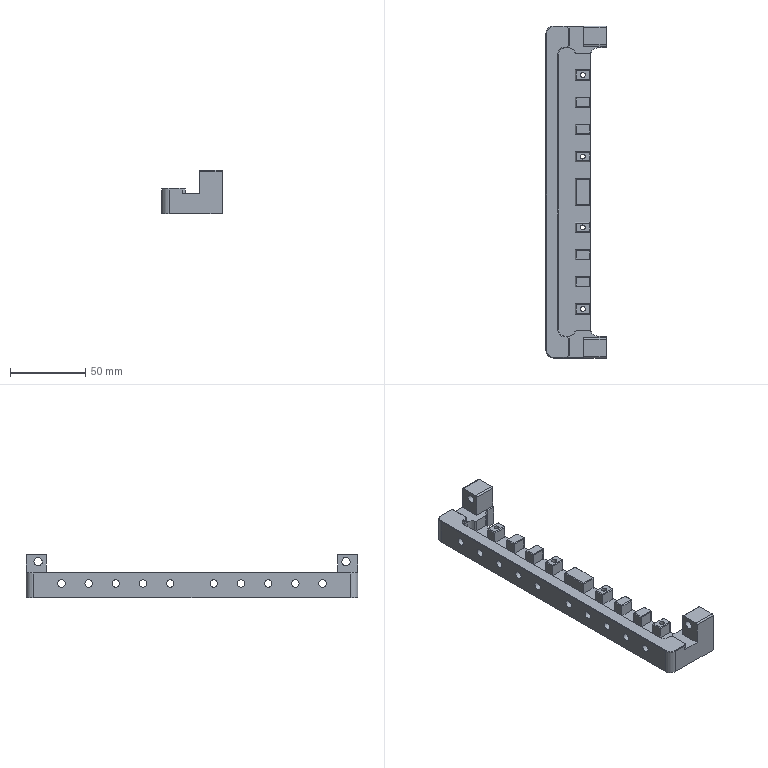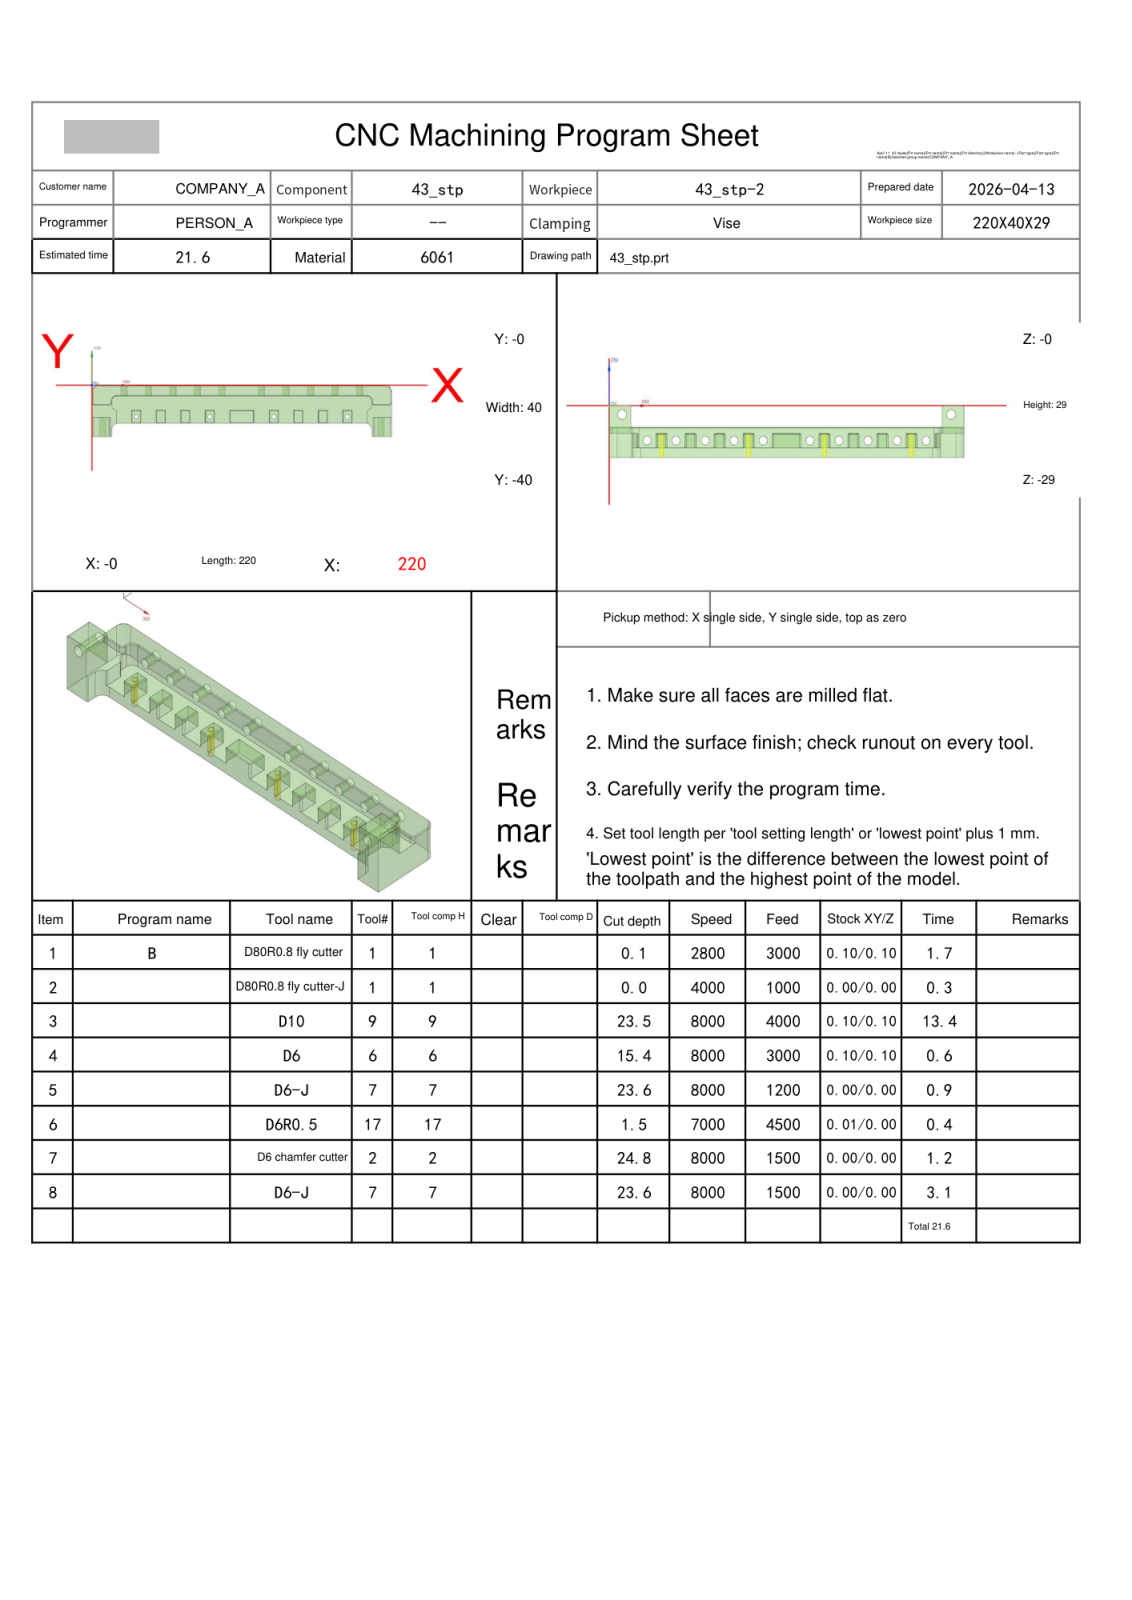NC program | NX | posted by the shop | part box 40 x 220 x 29 mm
Lines 8431 to 9376 of 14837:
N5 T07 M06
(D6-J  D=6. R=0. H=07 ce=0.00 di=0.00)
G00 G90 G54 X201.901 Y-14.131 M03 S8000
G43 H07 Z20.
M08
Z-12.147
G01 X201.908 Y-14.129 Z-12.238 F1200.
X201.93 Y-14.122 Z-12.32
X201.963 Y-14.111 Z-12.393
X202.006 Y-14.095 Z-12.458
X202.056 Y-14.074 Z-12.516
X202.112 Y-14.047 Z-12.565
X202.17 Y-14.014 Z-12.608
X202.23 Y-13.975 Z-12.644
X202.289 Y-13.929 Z-12.674
X202.345 Y-13.877 Z-12.698
X202.395 Y-13.817 Z-12.717
X202.438 Y-13.75 Z-12.73
X202.471 Y-13.675 Z-12.74
X202.492 Y-13.592 Z-12.745
X202.5 Y-13.5 Z-12.747
Y-12.5
G03 X201.5 Y-11.5 I-1. J0.0
G01 X200.434
X200.355 Y-11.516 Z-12.748
X200.299 Y-11.561 Z-12.75
X200.263 Y-11.632 Z-12.754
X200.246 Y-11.723 Z-12.76
X200.247 Y-11.833 Z-12.767
X200.263 Y-11.955 Z-12.774
X200.293 Y-12.087 Z-12.783
X200.336 Y-12.224 Z-12.793
X200.39 Y-12.363 Z-12.803
X200.453 Y-12.5 Z-12.813
X200.602 Y-12.754 Z-12.836
X200.78 Y-12.982 Z-12.858
X200.987 Y-13.183 Z-12.882
X201.221 Y-13.355 Z-12.904
X201.482 Y-13.498 Z-12.927
X201.621 Y-13.558 Z-12.937
X201.763 Y-13.609 Z-12.947
X201.903 Y-13.649 Z-12.957
X202.037 Y-13.677 Z-12.966
X202.162 Y-13.691 Z-12.973
X202.273 Y-13.69 Z-12.98
X202.366 Y-13.672 Z-12.986
X202.438 Y-13.635 Z-12.99
X202.484 Y-13.579 Z-12.992
X202.5 Y-13.5 Z-12.993
Y-12.5
G03 X201.5 Y-11.5 I-1. J0.0
G01 X200.434
X200.355 Y-11.516 Z-12.994
X200.299 Y-11.561 Z-12.997
X200.263 Y-11.632 Z-13.001
X200.246 Y-11.723 Z-13.006
X200.247 Y-11.833 Z-13.013
X200.263 Y-11.955 Z-13.021
X200.293 Y-12.087 Z-13.03
X200.336 Y-12.224 Z-13.039
X200.39 Y-12.363 Z-13.05
X200.453 Y-12.5 Z-13.06
X200.602 Y-12.754 Z-13.082
X200.78 Y-12.982 Z-13.105
X200.987 Y-13.183 Z-13.128
X201.221 Y-13.355 Z-13.151
X201.482 Y-13.498 Z-13.173
X201.621 Y-13.558 Z-13.184
X201.763 Y-13.609 Z-13.194
X201.903 Y-13.649 Z-13.203
X202.037 Y-13.677 Z-13.212
X202.162 Y-13.691 Z-13.22
X202.273 Y-13.69 Z-13.227
X202.366 Y-13.672 Z-13.232
X202.438 Y-13.635 Z-13.237
X202.484 Y-13.579 Z-13.239
X202.5 Y-13.5 Z-13.24
Y-12.5
G03 X201.5 Y-11.5 I-1. J0.0
G01 X200.434
X200.355 Y-11.516 Z-13.241
X200.299 Y-11.561 Z-13.243
X200.263 Y-11.632 Z-13.248
X200.246 Y-11.723 Z-13.253
X200.247 Y-11.833 Z-13.26
X200.263 Y-11.955 Z-13.268
X200.293 Y-12.087 Z-13.277
X200.336 Y-12.224 Z-13.286
X200.39 Y-12.363 Z-13.296
X200.453 Y-12.5 Z-13.307
X200.602 Y-12.754 Z-13.329
X200.78 Y-12.982 Z-13.352
X200.987 Y-13.183 Z-13.375
X201.221 Y-13.355 Z-13.398
X201.482 Y-13.498 Z-13.42
X201.621 Y-13.558 Z-13.43
X201.763 Y-13.609 Z-13.441
X201.903 Y-13.649 Z-13.45
X202.037 Y-13.677 Z-13.459
X202.162 Y-13.692 Z-13.467
X202.273 Y-13.69 Z-13.474
X202.366 Y-13.672 Z-13.479
X202.438 Y-13.635 Z-13.483
X202.484 Y-13.579 Z-13.486
X202.5 Y-13.5 Z-13.487
Y-12.5
G03 X201.5 Y-11.5 I-1. J0.0
G01 X200.434
X200.355 Y-11.516 Z-13.488
X200.299 Y-11.561 Z-13.49
X200.263 Y-11.632 Z-13.494
X200.246 Y-11.723 Z-13.5
X200.247 Y-11.833 Z-13.507
X200.263 Y-11.955 Z-13.514
X200.293 Y-12.087 Z-13.523
X200.336 Y-12.224 Z-13.533
X200.39 Y-12.363 Z-13.543
X200.453 Y-12.5 Z-13.553
X200.602 Y-12.754 Z-13.576
X200.78 Y-12.982 Z-13.598
X200.987 Y-13.183 Z-13.622
X201.221 Y-13.355 Z-13.644
X201.482 Y-13.498 Z-13.667
X201.621 Y-13.558 Z-13.677
X201.763 Y-13.609 Z-13.687
X201.903 Y-13.649 Z-13.697
X202.037 Y-13.677 Z-13.706
X202.162 Y-13.692 Z-13.713
X202.273 Y-13.69 Z-13.72
X202.366 Y-13.672 Z-13.726
X202.438 Y-13.635 Z-13.73
X202.484 Y-13.579 Z-13.732
X202.5 Y-13.5 Z-13.733
Y-12.5
G03 X201.5 Y-11.5 I-1. J0.0
G01 X200.434
X200.355 Y-11.516 Z-13.734
X200.299 Y-11.561 Z-13.737
X200.263 Y-11.632 Z-13.741
X200.246 Y-11.723 Z-13.746
X200.247 Y-11.833 Z-13.753
X200.263 Y-11.955 Z-13.761
X200.293 Y-12.087 Z-13.77
X200.336 Y-12.224 Z-13.779
X200.39 Y-12.363 Z-13.79
X200.453 Y-12.5 Z-13.8
X200.602 Y-12.754 Z-13.822
X200.78 Y-12.982 Z-13.845
X200.987 Y-13.183 Z-13.868
X201.221 Y-13.355 Z-13.891
X201.482 Y-13.498 Z-13.913
X201.621 Y-13.558 Z-13.924
X201.763 Y-13.609 Z-13.934
X201.903 Y-13.649 Z-13.943
X202.037 Y-13.677 Z-13.952
X202.162 Y-13.692 Z-13.96
X202.273 Y-13.69 Z-13.967
X202.366 Y-13.672 Z-13.972
X202.438 Y-13.635 Z-13.977
X202.484 Y-13.579 Z-13.979
X202.5 Y-13.5 Z-13.98
Y-12.5
G03 X201.5 Y-11.5 I-1. J0.0
G01 X200.434
X200.355 Y-11.516 Z-13.981
X200.299 Y-11.561 Z-13.983
X200.263 Y-11.632 Z-13.988
X200.246 Y-11.723 Z-13.993
X200.247 Y-11.833 Z-14.
X200.263 Y-11.955 Z-14.008
X200.293 Y-12.087 Z-14.017
X200.336 Y-12.224 Z-14.026
X200.39 Y-12.363 Z-14.036
X200.453 Y-12.5 Z-14.047
X200.602 Y-12.754 Z-14.069
X200.78 Y-12.982 Z-14.092
X200.987 Y-13.183 Z-14.115
X201.221 Y-13.355 Z-14.138
X201.482 Y-13.498 Z-14.16
X201.621 Y-13.558 Z-14.17
X201.763 Y-13.609 Z-14.181
X201.903 Y-13.649 Z-14.19
X202.037 Y-13.677 Z-14.199
X202.162 Y-13.692 Z-14.207
X202.273 Y-13.69 Z-14.214
X202.366 Y-13.672 Z-14.219
X202.438 Y-13.635 Z-14.223
X202.484 Y-13.579 Z-14.226
X202.5 Y-13.5 Z-14.227
Y-12.5
G03 X201.5 Y-11.5 I-1. J0.0
G01 X200.434
X200.355 Y-11.516 Z-14.228
X200.299 Y-11.561 Z-14.23
X200.263 Y-11.632 Z-14.234
X200.246 Y-11.723 Z-14.24
X200.247 Y-11.833 Z-14.247
X200.263 Y-11.955 Z-14.254
X200.293 Y-12.087 Z-14.263
X200.336 Y-12.224 Z-14.273
X200.39 Y-12.363 Z-14.283
X200.453 Y-12.5 Z-14.293
X200.602 Y-12.754 Z-14.316
X200.78 Y-12.982 Z-14.338
X200.987 Y-13.183 Z-14.362
X201.221 Y-13.355 Z-14.384
X201.482 Y-13.498 Z-14.407
X201.621 Y-13.558 Z-14.417
X201.763 Y-13.609 Z-14.427
X201.903 Y-13.649 Z-14.437
X202.037 Y-13.677 Z-14.446
X202.162 Y-13.692 Z-14.453
X202.273 Y-13.69 Z-14.46
X202.366 Y-13.672 Z-14.466
X202.438 Y-13.635 Z-14.47
X202.484 Y-13.579 Z-14.472
X202.5 Y-13.5 Z-14.473
Y-12.5
G03 X201.5 Y-11.5 I-1. J0.0
G01 X200.434
X200.355 Y-11.516 Z-14.474
X200.299 Y-11.561 Z-14.477
X200.263 Y-11.632 Z-14.481
X200.246 Y-11.723 Z-14.486
X200.247 Y-11.833 Z-14.493
X200.263 Y-11.955 Z-14.501
X200.293 Y-12.087 Z-14.51
X200.336 Y-12.224 Z-14.519
X200.39 Y-12.363 Z-14.53
X200.453 Y-12.5 Z-14.54
X200.602 Y-12.754 Z-14.562
X200.78 Y-12.982 Z-14.585
X200.987 Y-13.183 Z-14.608
X201.221 Y-13.355 Z-14.631
X201.482 Y-13.498 Z-14.653
X201.621 Y-13.558 Z-14.664
X201.763 Y-13.609 Z-14.674
X201.903 Y-13.649 Z-14.683
X202.037 Y-13.677 Z-14.692
X202.162 Y-13.692 Z-14.7
X202.273 Y-13.69 Z-14.707
X202.366 Y-13.672 Z-14.712
X202.438 Y-13.635 Z-14.717
X202.484 Y-13.579 Z-14.719
X202.5 Y-13.5 Z-14.72
Y-12.5
G03 X201.5 Y-11.5 I-1. J0.0
G01 X200.434
X200.355 Y-11.516 Z-14.721
X200.299 Y-11.561 Z-14.723
X200.263 Y-11.632 Z-14.728
X200.246 Y-11.723 Z-14.733
X200.247 Y-11.833 Z-14.74
X200.263 Y-11.955 Z-14.748
X200.293 Y-12.087 Z-14.757
X200.336 Y-12.224 Z-14.766
X200.39 Y-12.363 Z-14.776
X200.453 Y-12.5 Z-14.787
X200.602 Y-12.754 Z-14.809
X200.78 Y-12.982 Z-14.832
X200.987 Y-13.183 Z-14.855
X201.221 Y-13.355 Z-14.878
X201.482 Y-13.498 Z-14.9
X201.621 Y-13.558 Z-14.91
X201.763 Y-13.609 Z-14.921
X201.903 Y-13.649 Z-14.93
X202.037 Y-13.677 Z-14.939
X202.162 Y-13.692 Z-14.947
X202.273 Y-13.69 Z-14.954
X202.366 Y-13.672 Z-14.959
X202.438 Y-13.635 Z-14.963
X202.484 Y-13.579 Z-14.966
X202.5 Y-13.5 Z-14.967
Y-12.5
G03 X201.5 Y-11.5 I-1. J0.0
G01 X200.434
X200.355 Y-11.516 Z-14.968
X200.299 Y-11.561 Z-14.97
X200.263 Y-11.632 Z-14.974
X200.246 Y-11.723 Z-14.98
X200.247 Y-11.833 Z-14.987
X200.263 Y-11.955 Z-14.994
X200.293 Y-12.087 Z-15.003
X200.336 Y-12.224 Z-15.013
X200.39 Y-12.363 Z-15.023
X200.453 Y-12.5 Z-15.033
X200.602 Y-12.754 Z-15.056
X200.78 Y-12.982 Z-15.078
X200.987 Y-13.183 Z-15.102
X201.221 Y-13.355 Z-15.124
X201.482 Y-13.498 Z-15.147
X201.621 Y-13.558 Z-15.157
X201.763 Y-13.609 Z-15.167
X201.903 Y-13.649 Z-15.177
X202.037 Y-13.677 Z-15.186
X202.162 Y-13.692 Z-15.193
X202.273 Y-13.69 Z-15.2
X202.366 Y-13.672 Z-15.206
X202.438 Y-13.635 Z-15.21
X202.484 Y-13.579 Z-15.212
X202.5 Y-13.5 Z-15.213
Y-12.5
G03 X201.5 Y-11.5 I-1. J0.0
G01 X200.434
X200.355 Y-11.516 Z-15.214
X200.299 Y-11.561 Z-15.217
X200.263 Y-11.632 Z-15.221
X200.246 Y-11.723 Z-15.226
X200.247 Y-11.833 Z-15.233
X200.263 Y-11.955 Z-15.241
X200.293 Y-12.087 Z-15.25
X200.336 Y-12.224 Z-15.259
X200.39 Y-12.363 Z-15.27
X200.453 Y-12.5 Z-15.28
X200.602 Y-12.754 Z-15.302
X200.78 Y-12.982 Z-15.325
X200.987 Y-13.183 Z-15.348
X201.221 Y-13.355 Z-15.371
X201.482 Y-13.498 Z-15.393
X201.621 Y-13.558 Z-15.404
X201.763 Y-13.609 Z-15.414
X201.903 Y-13.649 Z-15.423
X202.037 Y-13.677 Z-15.432
X202.162 Y-13.692 Z-15.44
X202.273 Y-13.69 Z-15.447
X202.366 Y-13.672 Z-15.452
X202.438 Y-13.635 Z-15.457
X202.484 Y-13.579 Z-15.459
X202.5 Y-13.5 Z-15.46
Y-12.5
G03 X201.5 Y-11.5 I-1. J0.0
G01 X200.434
X200.355 Y-11.516 Z-15.461
X200.299 Y-11.562 Z-15.463
X200.263 Y-11.633 Z-15.468
X200.246 Y-11.725 Z-15.473
X200.247 Y-11.835 Z-15.48
X200.263 Y-11.959 Z-15.488
X200.293 Y-12.092 Z-15.497
X200.336 Y-12.231 Z-15.506
X200.389 Y-12.371 Z-15.516
X200.452 Y-12.509 Z-15.527
X200.601 Y-12.767 Z-15.549
X200.779 Y-12.999 Z-15.572
X200.985 Y-13.204 Z-15.595
X201.22 Y-13.382 Z-15.618
X201.481 Y-13.532 Z-15.64
X201.62 Y-13.596 Z-15.65
X201.762 Y-13.651 Z-15.661
X201.902 Y-13.696 Z-15.67
X202.037 Y-13.728 Z-15.679
X202.161 Y-13.746 Z-15.687
X202.273 Y-13.749 Z-15.694
X202.366 Y-13.734 Z-15.699
X202.438 Y-13.7 Z-15.703
X202.484 Y-13.644 Z-15.706
X202.5 Y-13.566 Z-15.707
Y-12.5
G03 X201.5 Y-11.5 I-1. J0.0
G01 X200.434
X200.355 Y-11.516 Z-15.708
X200.299 Y-11.562 Z-15.71
X200.263 Y-11.633 Z-15.714
X200.246 Y-11.725 Z-15.72
X200.247 Y-11.835 Z-15.727
X200.263 Y-11.959 Z-15.734
X200.293 Y-12.092 Z-15.743
X200.336 Y-12.231 Z-15.753
X200.389 Y-12.371 Z-15.763
X200.452 Y-12.509 Z-15.773
X200.601 Y-12.767 Z-15.796
X200.779 Y-12.999 Z-15.818
X200.985 Y-13.204 Z-15.842
X201.22 Y-13.382 Z-15.864
X201.481 Y-13.532 Z-15.887
X201.62 Y-13.596 Z-15.897
X201.762 Y-13.651 Z-15.907
X201.902 Y-13.696 Z-15.917
X202.037 Y-13.728 Z-15.926
X202.161 Y-13.746 Z-15.933
X202.273 Y-13.749 Z-15.94
X202.366 Y-13.734 Z-15.946
X202.438 Y-13.7 Z-15.95
X202.484 Y-13.644 Z-15.952
X202.5 Y-13.566 Z-15.953
Y-12.5
G03 X201.5 Y-11.5 I-1. J0.0
G01 X200.434
X200.355 Y-11.516 Z-15.954
X200.299 Y-11.562 Z-15.957
X200.263 Y-11.633 Z-15.961
X200.246 Y-11.725 Z-15.966
X200.247 Y-11.835 Z-15.973
X200.263 Y-11.959 Z-15.981
X200.293 Y-12.092 Z-15.99
X200.336 Y-12.231 Z-15.999
X200.389 Y-12.371 Z-16.01
X200.452 Y-12.509 Z-16.02
X200.601 Y-12.767 Z-16.042
X200.779 Y-12.999 Z-16.065
X200.985 Y-13.204 Z-16.088
X201.22 Y-13.382 Z-16.111
X201.481 Y-13.532 Z-16.133
X201.62 Y-13.596 Z-16.144
X201.762 Y-13.651 Z-16.154
X201.902 Y-13.696 Z-16.163
X202.037 Y-13.728 Z-16.172
X202.161 Y-13.746 Z-16.18
X202.273 Y-13.749 Z-16.187
X202.366 Y-13.734 Z-16.192
X202.438 Y-13.7 Z-16.197
X202.484 Y-13.644 Z-16.199
X202.5 Y-13.566 Z-16.2
Y-12.5
G03 X201.5 Y-11.5 I-1. J0.0
G01 X200.434
X200.355 Y-11.516 Z-16.201
X200.299 Y-11.562 Z-16.203
X200.263 Y-11.633 Z-16.208
X200.246 Y-11.725 Z-16.213
X200.247 Y-11.835 Z-16.22
X200.263 Y-11.959 Z-16.228
X200.293 Y-12.092 Z-16.237
X200.336 Y-12.231 Z-16.246
X200.389 Y-12.371 Z-16.256
X200.452 Y-12.509 Z-16.267
X200.601 Y-12.767 Z-16.289
X200.779 Y-12.999 Z-16.312
X200.985 Y-13.204 Z-16.335
X201.22 Y-13.382 Z-16.358
X201.481 Y-13.532 Z-16.38
X201.62 Y-13.596 Z-16.39
X201.762 Y-13.651 Z-16.401
X201.902 Y-13.696 Z-16.41
X202.037 Y-13.728 Z-16.419
X202.161 Y-13.746 Z-16.427
X202.273 Y-13.749 Z-16.434
X202.366 Y-13.734 Z-16.439
X202.438 Y-13.7 Z-16.443
X202.484 Y-13.644 Z-16.446
X202.5 Y-13.566 Z-16.447
Y-12.5
G03 X201.5 Y-11.5 I-1. J0.0
G01 X200.434
X200.355 Y-11.516 Z-16.448
X200.299 Y-11.562 Z-16.45
X200.263 Y-11.633 Z-16.454
X200.246 Y-11.725 Z-16.46
X200.247 Y-11.835 Z-16.467
X200.263 Y-11.959 Z-16.474
X200.293 Y-12.092 Z-16.483
X200.336 Y-12.231 Z-16.493
X200.389 Y-12.371 Z-16.503
X200.452 Y-12.509 Z-16.513
X200.601 Y-12.767 Z-16.536
X200.779 Y-12.999 Z-16.558
X200.985 Y-13.204 Z-16.582
X201.22 Y-13.382 Z-16.604
X201.481 Y-13.532 Z-16.627
X201.62 Y-13.596 Z-16.637
X201.762 Y-13.651 Z-16.647
X201.902 Y-13.696 Z-16.657
X202.037 Y-13.728 Z-16.666
X202.161 Y-13.746 Z-16.673
X202.273 Y-13.749 Z-16.68
X202.366 Y-13.734 Z-16.686
X202.438 Y-13.7 Z-16.69
X202.484 Y-13.644 Z-16.692
X202.5 Y-13.566 Z-16.693
Y-12.5
G03 X201.5 Y-11.5 I-1. J0.0
G01 X200.434
X200.355 Y-11.516 Z-16.694
X200.299 Y-11.562 Z-16.697
X200.263 Y-11.633 Z-16.701
X200.246 Y-11.725 Z-16.706
X200.247 Y-11.835 Z-16.713
X200.263 Y-11.959 Z-16.721
X200.293 Y-12.092 Z-16.73
X200.336 Y-12.231 Z-16.739
X200.389 Y-12.371 Z-16.75
X200.452 Y-12.509 Z-16.76
X200.601 Y-12.767 Z-16.782
X200.779 Y-12.999 Z-16.805
X200.985 Y-13.204 Z-16.828
X201.22 Y-13.382 Z-16.851
X201.481 Y-13.532 Z-16.873
X201.62 Y-13.596 Z-16.884
X201.762 Y-13.651 Z-16.894
X201.902 Y-13.696 Z-16.903
X202.037 Y-13.728 Z-16.912
X202.161 Y-13.746 Z-16.92
X202.273 Y-13.749 Z-16.927
X202.366 Y-13.734 Z-16.932
X202.438 Y-13.7 Z-16.937
X202.484 Y-13.644 Z-16.939
X202.5 Y-13.566 Z-16.94
Y-12.5
G03 X201.5 Y-11.5 I-1. J0.0
G01 X200.434
X200.355 Y-11.516 Z-16.941
X200.299 Y-11.562 Z-16.943
X200.263 Y-11.633 Z-16.948
X200.246 Y-11.725 Z-16.953
X200.247 Y-11.835 Z-16.96
X200.263 Y-11.959 Z-16.968
X200.293 Y-12.092 Z-16.977
X200.336 Y-12.231 Z-16.986
X200.389 Y-12.371 Z-16.996
X200.452 Y-12.509 Z-17.007
X200.601 Y-12.767 Z-17.029
X200.779 Y-12.999 Z-17.052
X200.985 Y-13.204 Z-17.075
X201.22 Y-13.382 Z-17.098
X201.481 Y-13.532 Z-17.12
X201.62 Y-13.596 Z-17.13
X201.762 Y-13.651 Z-17.141
X201.902 Y-13.696 Z-17.15
X202.037 Y-13.728 Z-17.159
X202.161 Y-13.746 Z-17.167
X202.273 Y-13.749 Z-17.174
X202.366 Y-13.734 Z-17.179
X202.438 Y-13.7 Z-17.183
X202.484 Y-13.644 Z-17.186
X202.5 Y-13.566 Z-17.187
Y-12.5
G03 X201.5 Y-11.5 I-1. J0.0
G01 X200.434
X200.355 Y-11.516 Z-17.188
X200.299 Y-11.562 Z-17.19
X200.263 Y-11.633 Z-17.194
X200.246 Y-11.725 Z-17.2
X200.247 Y-11.835 Z-17.207
X200.263 Y-11.959 Z-17.214
X200.293 Y-12.092 Z-17.223
X200.336 Y-12.231 Z-17.233
X200.389 Y-12.371 Z-17.243
X200.452 Y-12.509 Z-17.253
X200.601 Y-12.767 Z-17.276
X200.779 Y-12.999 Z-17.298
X200.985 Y-13.204 Z-17.322
X201.22 Y-13.382 Z-17.344
X201.481 Y-13.532 Z-17.367
X201.62 Y-13.596 Z-17.377
X201.762 Y-13.651 Z-17.387
X201.902 Y-13.696 Z-17.397
X202.037 Y-13.728 Z-17.406
X202.161 Y-13.746 Z-17.413
X202.273 Y-13.749 Z-17.42
X202.366 Y-13.734 Z-17.426
X202.438 Y-13.7 Z-17.43
X202.484 Y-13.644 Z-17.432
X202.5 Y-13.566 Z-17.433
Y-12.5
G03 X201.5 Y-11.5 I-1. J0.0
G01 X200.434
X200.355 Y-11.516 Z-17.434
X200.299 Y-11.562 Z-17.437
X200.263 Y-11.633 Z-17.441
X200.246 Y-11.725 Z-17.446
X200.247 Y-11.835 Z-17.453
X200.263 Y-11.959 Z-17.461
X200.293 Y-12.092 Z-17.47
X200.336 Y-12.231 Z-17.479
X200.389 Y-12.371 Z-17.49
X200.452 Y-12.509 Z-17.5
X200.601 Y-12.767 Z-17.522
X200.779 Y-12.999 Z-17.545
X200.985 Y-13.204 Z-17.568
X201.22 Y-13.382 Z-17.591
X201.481 Y-13.532 Z-17.613
X201.62 Y-13.596 Z-17.624
X201.762 Y-13.651 Z-17.634
X201.902 Y-13.696 Z-17.643
X202.037 Y-13.728 Z-17.652
X202.161 Y-13.746 Z-17.66
X202.273 Y-13.749 Z-17.667
X202.366 Y-13.734 Z-17.672
X202.438 Y-13.7 Z-17.677
X202.484 Y-13.644 Z-17.679
X202.5 Y-13.566 Z-17.68
Y-12.5
G03 X201.5 Y-11.5 I-1. J0.0
G01 X200.434
X200.355 Y-11.516 Z-17.681
X200.299 Y-11.562 Z-17.683
X200.263 Y-11.633 Z-17.688
X200.246 Y-11.725 Z-17.693
X200.247 Y-11.835 Z-17.7
X200.263 Y-11.959 Z-17.708
X200.293 Y-12.092 Z-17.717
X200.336 Y-12.231 Z-17.726
X200.389 Y-12.371 Z-17.736
X200.452 Y-12.509 Z-17.747
X200.601 Y-12.767 Z-17.769
X200.779 Y-12.999 Z-17.792
X200.985 Y-13.204 Z-17.815
X201.22 Y-13.382 Z-17.838
X201.481 Y-13.532 Z-17.86
X201.62 Y-13.596 Z-17.87
X201.762 Y-13.651 Z-17.881
X201.902 Y-13.696 Z-17.89
X202.037 Y-13.728 Z-17.899
X202.161 Y-13.746 Z-17.907
X202.273 Y-13.749 Z-17.914
X202.366 Y-13.734 Z-17.919
X202.438 Y-13.7 Z-17.923
X202.484 Y-13.644 Z-17.926
X202.5 Y-13.566 Z-17.927
Y-12.5
G03 X201.5 Y-11.5 I-1. J0.0
G01 X200.434
X200.355 Y-11.516 Z-17.928
X200.299 Y-11.562 Z-17.93
X200.263 Y-11.633 Z-17.934
X200.246 Y-11.725 Z-17.94
X200.247 Y-11.835 Z-17.947
X200.263 Y-11.959 Z-17.954
X200.293 Y-12.092 Z-17.963
X200.336 Y-12.231 Z-17.973
X200.389 Y-12.371 Z-17.983
X200.452 Y-12.509 Z-17.993
X200.601 Y-12.767 Z-18.016
X200.779 Y-12.999 Z-18.038
X200.985 Y-13.204 Z-18.062
X201.22 Y-13.382 Z-18.084
X201.481 Y-13.532 Z-18.107
X201.62 Y-13.596 Z-18.117
X201.762 Y-13.651 Z-18.127
X201.902 Y-13.696 Z-18.137
X202.037 Y-13.728 Z-18.146
X202.161 Y-13.746 Z-18.153
X202.273 Y-13.749 Z-18.16
X202.366 Y-13.734 Z-18.166
X202.438 Y-13.7 Z-18.17
X202.484 Y-13.644 Z-18.172
X202.5 Y-13.566 Z-18.173
Y-12.5
G03 X201.5 Y-11.5 I-1. J0.0
G01 X200.434
X200.355 Y-11.516 Z-18.174
X200.299 Y-11.562 Z-18.177
X200.263 Y-11.633 Z-18.181
X200.246 Y-11.725 Z-18.186
X200.247 Y-11.835 Z-18.193
X200.263 Y-11.959 Z-18.201
X200.293 Y-12.092 Z-18.21
X200.336 Y-12.231 Z-18.219
X200.389 Y-12.371 Z-18.23
X200.452 Y-12.509 Z-18.24
X200.601 Y-12.767 Z-18.262
X200.779 Y-12.999 Z-18.285
X200.985 Y-13.204 Z-18.308
X201.22 Y-13.382 Z-18.331
X201.481 Y-13.532 Z-18.353
X201.62 Y-13.596 Z-18.364
X201.762 Y-13.651 Z-18.374
X201.902 Y-13.696 Z-18.383
X202.037 Y-13.728 Z-18.392
X202.161 Y-13.746 Z-18.4
X202.273 Y-13.749 Z-18.407
X202.366 Y-13.734 Z-18.412
X202.438 Y-13.7 Z-18.417
X202.484 Y-13.644 Z-18.419
X202.5 Y-13.566 Z-18.42
Y-12.5
G03 X201.5 Y-11.5 I-1. J0.0
G01 X200.434
X200.355 Y-11.516 Z-18.421
X200.299 Y-11.562 Z-18.423
X200.263 Y-11.633 Z-18.428
X200.246 Y-11.725 Z-18.433
X200.247 Y-11.835 Z-18.44
X200.263 Y-11.959 Z-18.448
X200.293 Y-12.092 Z-18.457
X200.336 Y-12.231 Z-18.466
X200.389 Y-12.371 Z-18.476
X200.452 Y-12.509 Z-18.487
X200.601 Y-12.767 Z-18.509
X200.779 Y-12.999 Z-18.532
X200.985 Y-13.204 Z-18.555
X201.22 Y-13.382 Z-18.578
X201.481 Y-13.532 Z-18.6
X201.62 Y-13.596 Z-18.61
X201.762 Y-13.651 Z-18.621
X201.902 Y-13.696 Z-18.63
X202.037 Y-13.728 Z-18.639
X202.161 Y-13.746 Z-18.647
X202.273 Y-13.749 Z-18.654
X202.366 Y-13.734 Z-18.659
X202.438 Y-13.7 Z-18.663
X202.484 Y-13.644 Z-18.666
X202.5 Y-13.566 Z-18.667
Y-12.5
G03 X201.5 Y-11.5 I-1. J0.0
G01 X200.434
X200.355 Y-11.516 Z-18.668
X200.299 Y-11.562 Z-18.67
X200.263 Y-11.633 Z-18.674
X200.246 Y-11.725 Z-18.68
X200.247 Y-11.835 Z-18.687
X200.263 Y-11.959 Z-18.694
X200.293 Y-12.092 Z-18.703
X200.336 Y-12.231 Z-18.713
X200.389 Y-12.371 Z-18.723
X200.452 Y-12.509 Z-18.733
X200.601 Y-12.767 Z-18.756
X200.779 Y-12.999 Z-18.778
X200.985 Y-13.204 Z-18.802
X201.22 Y-13.382 Z-18.824
X201.481 Y-13.532 Z-18.847
X201.62 Y-13.596 Z-18.857
X201.762 Y-13.651 Z-18.867
X201.902 Y-13.696 Z-18.877
X202.037 Y-13.728 Z-18.886
X202.161 Y-13.746 Z-18.893
X202.273 Y-13.749 Z-18.9
X202.366 Y-13.734 Z-18.906
X202.438 Y-13.7 Z-18.91
X202.484 Y-13.644 Z-18.912
X202.5 Y-13.566 Z-18.913
Y-12.5
G03 X201.5 Y-11.5 I-1. J0.0
G01 X200.434
X200.355 Y-11.516 Z-18.914
X200.299 Y-11.562 Z-18.917
X200.263 Y-11.633 Z-18.921
X200.246 Y-11.725 Z-18.926
X200.247 Y-11.835 Z-18.933
X200.263 Y-11.959 Z-18.941
X200.293 Y-12.092 Z-18.95
X200.336 Y-12.231 Z-18.959
X200.389 Y-12.371 Z-18.97
X200.452 Y-12.509 Z-18.98
X200.601 Y-12.767 Z-19.002
X200.779 Y-12.999 Z-19.025
X200.985 Y-13.204 Z-19.048
X201.22 Y-13.382 Z-19.071
X201.481 Y-13.532 Z-19.093
X201.62 Y-13.596 Z-19.104
X201.762 Y-13.651 Z-19.114
X201.902 Y-13.696 Z-19.123
X202.037 Y-13.728 Z-19.132
X202.161 Y-13.746 Z-19.14
X202.273 Y-13.749 Z-19.147
X202.366 Y-13.734 Z-19.152
X202.438 Y-13.7 Z-19.157
X202.484 Y-13.644 Z-19.159
X202.5 Y-13.566 Z-19.16
Y-12.5
G03 X201.5 Y-11.5 I-1. J0.0
G01 X200.434
X200.355 Y-11.516 Z-19.161
X200.299 Y-11.562 Z-19.163
X200.263 Y-11.633 Z-19.168
X200.246 Y-11.725 Z-19.173
X200.247 Y-11.835 Z-19.18
X200.263 Y-11.959 Z-19.188
X200.293 Y-12.092 Z-19.197
X200.336 Y-12.231 Z-19.206
X200.389 Y-12.371 Z-19.216
X200.452 Y-12.509 Z-19.227
X200.601 Y-12.767 Z-19.249
X200.779 Y-12.999 Z-19.272
X200.985 Y-13.204 Z-19.295
X201.22 Y-13.382 Z-19.318
X201.481 Y-13.532 Z-19.34
X201.62 Y-13.596 Z-19.35
X201.762 Y-13.651 Z-19.361
X201.902 Y-13.696 Z-19.37
X202.037 Y-13.728 Z-19.379
X202.161 Y-13.746 Z-19.387
X202.273 Y-13.749 Z-19.394
X202.366 Y-13.734 Z-19.399
X202.438 Y-13.7 Z-19.403
X202.484 Y-13.644 Z-19.406
X202.5 Y-13.566 Z-19.407
Y-12.5
G03 X201.5 Y-11.5 I-1. J0.0
G01 X200.434
X200.355 Y-11.516 Z-19.408
X200.299 Y-11.562 Z-19.41
X200.263 Y-11.633 Z-19.414
X200.246 Y-11.725 Z-19.42
X200.247 Y-11.835 Z-19.427
X200.263 Y-11.959 Z-19.434
X200.293 Y-12.092 Z-19.443
X200.336 Y-12.231 Z-19.453
X200.389 Y-12.371 Z-19.463
X200.452 Y-12.509 Z-19.473
X200.601 Y-12.767 Z-19.496
X200.779 Y-12.999 Z-19.518
X200.985 Y-13.204 Z-19.542
X201.22 Y-13.382 Z-19.564
X201.481 Y-13.532 Z-19.587
X201.62 Y-13.596 Z-19.597
X201.762 Y-13.651 Z-19.607
X201.902 Y-13.696 Z-19.617
X202.037 Y-13.728 Z-19.626
X202.161 Y-13.746 Z-19.633
X202.273 Y-13.749 Z-19.64
X202.366 Y-13.734 Z-19.646
X202.438 Y-13.7 Z-19.65
X202.484 Y-13.644 Z-19.652
X202.5 Y-13.566 Z-19.653
Y-12.5
G03 X201.5 Y-11.5 I-1. J0.0
G01 X200.434
X200.355 Y-11.516 Z-19.654
X200.299 Y-11.562 Z-19.657
X200.263 Y-11.633 Z-19.661
X200.246 Y-11.725 Z-19.666
X200.247 Y-11.835 Z-19.673
X200.263 Y-11.959 Z-19.681
X200.293 Y-12.092 Z-19.69
X200.336 Y-12.231 Z-19.699
X200.389 Y-12.371 Z-19.71
X200.452 Y-12.509 Z-19.72
X200.601 Y-12.767 Z-19.742
X200.779 Y-12.999 Z-19.765
X200.985 Y-13.204 Z-19.788
X201.22 Y-13.382 Z-19.811
X201.481 Y-13.532 Z-19.833
X201.62 Y-13.596 Z-19.844
X201.762 Y-13.651 Z-19.854
X201.902 Y-13.696 Z-19.863
X202.037 Y-13.728 Z-19.872
X202.161 Y-13.746 Z-19.88
X202.273 Y-13.749 Z-19.887
X202.366 Y-13.734 Z-19.892
X202.438 Y-13.7 Z-19.897
X202.484 Y-13.644 Z-19.899
X202.5 Y-13.566 Z-19.9
Y-12.5
G03 X201.5 Y-11.5 I-1. J0.0
G01 X200.434
X200.355 Y-11.516 Z-19.901
X200.299 Y-11.562 Z-19.903
X200.263 Y-11.633 Z-19.908
X200.246 Y-11.725 Z-19.913
X200.247 Y-11.835 Z-19.92
X200.263 Y-11.959 Z-19.928
X200.293 Y-12.092 Z-19.937
X200.336 Y-12.231 Z-19.946
X200.389 Y-12.371 Z-19.956
X200.452 Y-12.509 Z-19.967
X200.601 Y-12.767 Z-19.989
X200.779 Y-12.999 Z-20.012
X200.985 Y-13.204 Z-20.035
X201.22 Y-13.382 Z-20.058
X201.481 Y-13.532 Z-20.08
X201.62 Y-13.596 Z-20.09
X201.762 Y-13.651 Z-20.101
X201.902 Y-13.696 Z-20.11
X202.037 Y-13.728 Z-20.119
X202.161 Y-13.746 Z-20.127
X202.273 Y-13.749 Z-20.134
X202.366 Y-13.734 Z-20.139
X202.438 Y-13.7 Z-20.143
X202.484 Y-13.644 Z-20.146
X202.5 Y-13.566 Z-20.147
Y-12.5
G03 X201.5 Y-11.5 I-1. J0.0
G01 X200.434
X200.355 Y-11.516 Z-20.148
X200.299 Y-11.562 Z-20.15
X200.263 Y-11.633 Z-20.154
X200.246 Y-11.725 Z-20.16
X200.247 Y-11.835 Z-20.167
X200.263 Y-11.959 Z-20.174
X200.293 Y-12.092 Z-20.183
X200.336 Y-12.231 Z-20.193
X200.389 Y-12.371 Z-20.203
X200.452 Y-12.509 Z-20.213
X200.601 Y-12.767 Z-20.236
X200.779 Y-12.999 Z-20.258
X200.985 Y-13.204 Z-20.282
X201.22 Y-13.382 Z-20.304
X201.481 Y-13.532 Z-20.327
X201.62 Y-13.596 Z-20.337
X201.762 Y-13.651 Z-20.347
X201.902 Y-13.696 Z-20.357
X202.037 Y-13.728 Z-20.366
X202.161 Y-13.746 Z-20.373
X202.273 Y-13.749 Z-20.38
X202.366 Y-13.734 Z-20.386
X202.438 Y-13.7 Z-20.39
X202.484 Y-13.644 Z-20.392
X202.5 Y-13.566 Z-20.393
Y-12.5
G03 X201.5 Y-11.5 I-1. J0.0
G01 X200.434
X200.355 Y-11.516 Z-20.394
X200.299 Y-11.562 Z-20.397
X200.263 Y-11.633 Z-20.401
X200.246 Y-11.725 Z-20.406
X200.247 Y-11.835 Z-20.413
X200.263 Y-11.959 Z-20.421
X200.293 Y-12.092 Z-20.43
X200.336 Y-12.231 Z-20.439
X200.389 Y-12.371 Z-20.45
X200.452 Y-12.509 Z-20.46
X200.601 Y-12.767 Z-20.482
X200.779 Y-12.999 Z-20.505
X200.985 Y-13.204 Z-20.528
X201.22 Y-13.382 Z-20.551
X201.481 Y-13.532 Z-20.573
X201.62 Y-13.596 Z-20.584
X201.762 Y-13.651 Z-20.594
X201.902 Y-13.696 Z-20.603
X202.037 Y-13.728 Z-20.612
X202.161 Y-13.746 Z-20.62
X202.273 Y-13.749 Z-20.627
X202.366 Y-13.734 Z-20.632
X202.438 Y-13.7 Z-20.637
X202.484 Y-13.644 Z-20.639
X202.5 Y-13.566 Z-20.64
Y-12.5
G03 X201.5 Y-11.5 I-1. J0.0
G01 X200.434
X200.355 Y-11.516 Z-20.641
X200.299 Y-11.562 Z-20.643
X200.263 Y-11.633 Z-20.648
X200.246 Y-11.725 Z-20.653
X200.247 Y-11.835 Z-20.66
X200.263 Y-11.959 Z-20.668
X200.293 Y-12.092 Z-20.677
X200.336 Y-12.231 Z-20.686
X200.389 Y-12.371 Z-20.696
X200.452 Y-12.509 Z-20.707
X200.601 Y-12.767 Z-20.729
X200.779 Y-12.999 Z-20.752
X200.985 Y-13.204 Z-20.775
X201.22 Y-13.382 Z-20.798
X201.481 Y-13.532 Z-20.82
X201.62 Y-13.596 Z-20.83
X201.762 Y-13.651 Z-20.841
X201.902 Y-13.696 Z-20.85
X202.037 Y-13.728 Z-20.859
X202.161 Y-13.746 Z-20.867
X202.273 Y-13.749 Z-20.874
X202.366 Y-13.734 Z-20.879
X202.438 Y-13.7 Z-20.883
X202.484 Y-13.644 Z-20.886
X202.5 Y-13.566 Z-20.887
Y-12.5